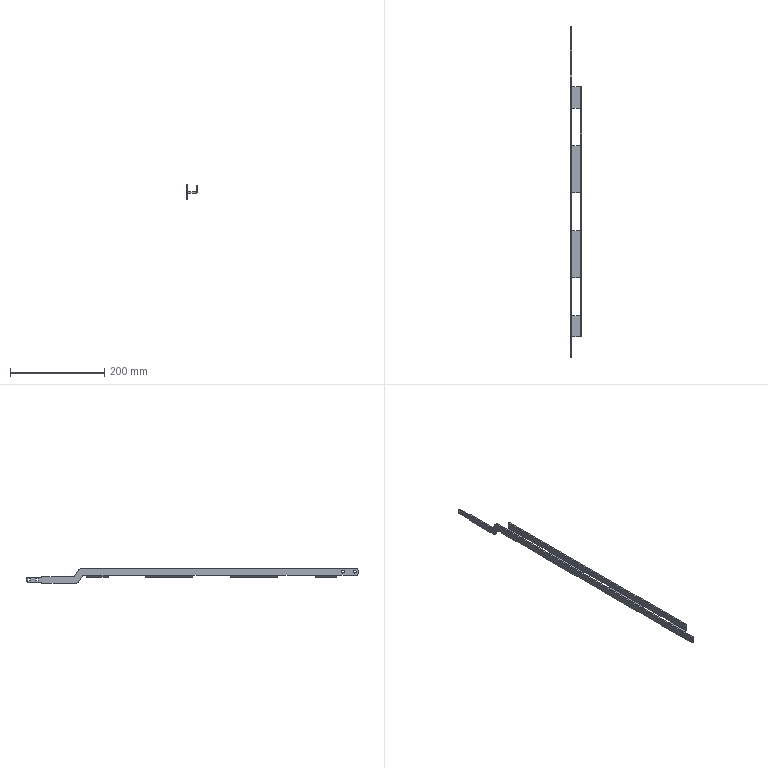Part | SolidWorks | features BaseBody 1 | 1 solid | 85 faces | box 25 x 704 x 30.5 mm | volume 71696 mm3 | plane 57 | cylinder 28 | commonest cylinder face diameters 6 x10 1 x8 7 x8 20 x2